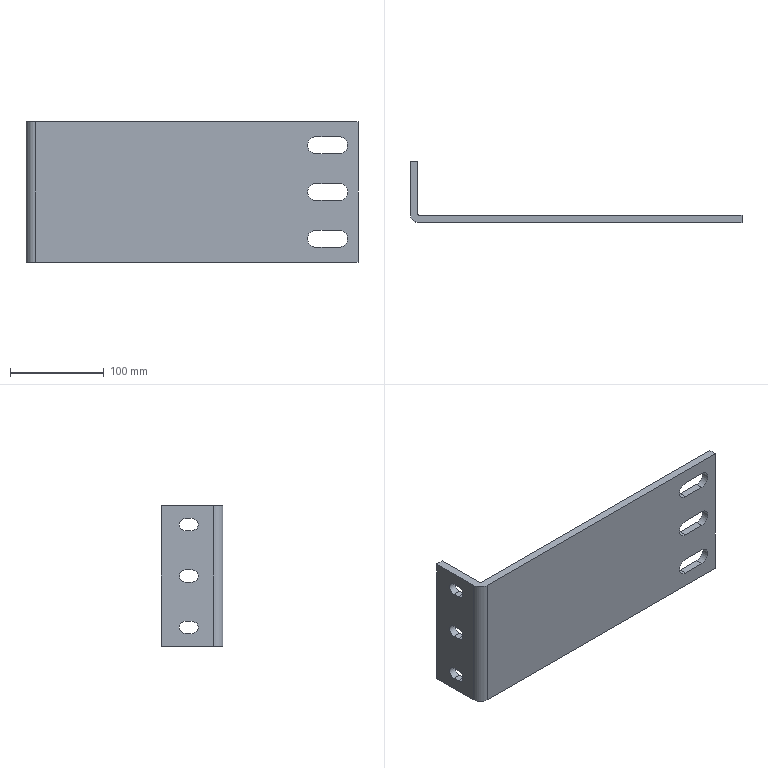Part | SolidWorks | features ICE 2, Extrusion 1 | 1 solid | 34 faces | box 355 x 66 x 150 mm | volume 470233 mm3 | plane 20 | cylinder 14 | commonest cylinder face diameters 13 x6 18 x6 4 x1 20 x1
STEP:
#1=CARTESIAN_POINT('',(8.,0.,0.));
#2=VERTEX_POINT('',#1);
#3=CARTESIAN_POINT('',(0.,0.,0.));
#4=VERTEX_POINT('',#3);
#5=CARTESIAN_POINT('',(8.,0.,0.));
#6=DIRECTION('',(-1.,0.,0.));
#7=VECTOR('',#6,1000.);
#8=LINE('',#5,#7);
#9=EDGE_CURVE('',#2,#4,#8,.T.);
#10=ORIENTED_EDGE('',*,*,#9,.T.);
#11=CARTESIAN_POINT('',(0.,0.,150.));
#12=VERTEX_POINT('',#11);
#13=CARTESIAN_POINT('',(0.,0.,150.));
#14=DIRECTION('',(0.,0.,-1.));
#15=VECTOR('',#14,1000.);
#16=LINE('',#13,#15);
#17=EDGE_CURVE('',#12,#4,#16,.T.);
#18=ORIENTED_EDGE('',*,*,#17,.F.);
#19=CARTESIAN_POINT('',(8.,0.,150.));
#20=VERTEX_POINT('',#19);
#21=CARTESIAN_POINT('',(8.,0.,150.));
#22=DIRECTION('',(-1.,0.,0.));
#23=VECTOR('',#22,1000.);
#24=LINE('',#21,#23);
#25=EDGE_CURVE('',#20,#12,#24,.T.);
#26=ORIENTED_EDGE('',*,*,#25,.F.);
#27=CARTESIAN_POINT('',(8.,0.,150.));
#28=DIRECTION('',(0.,0.,-1.));
#29=VECTOR('',#28,1000.);
#30=LINE('',#27,#29);
#31=EDGE_CURVE('',#20,#2,#30,.T.);
#32=ORIENTED_EDGE('',*,*,#31,.T.);
#33=EDGE_LOOP('',(#10,#18,#26,#32));
#34=FACE_OUTER_BOUND('',#33,.T.);
#35=CARTESIAN_POINT('',(8.,0.,150.));
#36=DIRECTION('',(0.,-1.,0.));
#37=DIRECTION('',(0.,0.,-1.));
#38=AXIS2_PLACEMENT_3D('',#35,#36,#37);
#39=PLANE('',#38);
#40=ADVANCED_FACE('',(#34),#39,.F.);
#41=CARTESIAN_POINT('',(0.,-26.,13.5));
#42=VERTEX_POINT('',#41);
#43=CARTESIAN_POINT('',(0.,-33.,13.5));
#44=VERTEX_POINT('',#43);
#45=CARTESIAN_POINT('',(0.,-26.,13.5));
#46=DIRECTION('',(0.,-1.,0.));
#47=VECTOR('',#46,1000.);
#48=LINE('',#45,#47);
#49=EDGE_CURVE('',#42,#44,#48,.T.);
#50=ORIENTED_EDGE('',*,*,#49,.F.);
#51=CARTESIAN_POINT('',(0.,-26.,26.5));
#52=VERTEX_POINT('',#51);
#53=CARTESIAN_POINT('',(0.,-26.,20.));
#54=DIRECTION('',(-1.,0.,0.));
#55=DIRECTION('',(0.,0.,1.));
#56=AXIS2_PLACEMENT_3D('',#53,#54,#55);
#57=CIRCLE('',#56,6.5);
#58=EDGE_CURVE('',#52,#42,#57,.T.);
#59=ORIENTED_EDGE('',*,*,#58,.F.);
#60=CARTESIAN_POINT('',(0.,-33.,26.5));
#61=VERTEX_POINT('',#60);
#62=CARTESIAN_POINT('',(0.,-26.,26.5));
#63=DIRECTION('',(0.,1.,0.));
#64=VECTOR('',#63,1000.);
#65=LINE('',#62,#64);
#66=EDGE_CURVE('',#61,#52,#65,.T.);
#67=ORIENTED_EDGE('',*,*,#66,.F.);
#68=CARTESIAN_POINT('',(0.,-33.,20.));
#69=DIRECTION('',(-1.,0.,0.));
#70=DIRECTION('',(0.,0.,1.));
#71=AXIS2_PLACEMENT_3D('',#68,#69,#70);
#72=CIRCLE('',#71,6.5);
#73=EDGE_CURVE('',#44,#61,#72,.T.);
#74=ORIENTED_EDGE('',*,*,#73,.F.);
#75=EDGE_LOOP('',(#50,#59,#67,#74));
#76=FACE_BOUND('',#75,.T.);
#77=CARTESIAN_POINT('',(0.,-26.,68.5));
#78=VERTEX_POINT('',#77);
#79=CARTESIAN_POINT('',(0.,-33.,68.5));
#80=VERTEX_POINT('',#79);
#81=CARTESIAN_POINT('',(0.,-26.,68.5));
#82=DIRECTION('',(0.,-1.,0.));
#83=VECTOR('',#82,1000.);
#84=LINE('',#81,#83);
#85=EDGE_CURVE('',#78,#80,#84,.T.);
#86=ORIENTED_EDGE('',*,*,#85,.F.);
#87=CARTESIAN_POINT('',(0.,-26.,81.5));
#88=VERTEX_POINT('',#87);
#89=CARTESIAN_POINT('',(0.,-26.,75.));
#90=DIRECTION('',(-1.,0.,0.));
#91=DIRECTION('',(0.,0.,1.));
#92=AXIS2_PLACEMENT_3D('',#89,#90,#91);
#93=CIRCLE('',#92,6.5);
#94=EDGE_CURVE('',#88,#78,#93,.T.);
#95=ORIENTED_EDGE('',*,*,#94,.F.);
#96=CARTESIAN_POINT('',(0.,-33.,81.5));
#97=VERTEX_POINT('',#96);
#98=CARTESIAN_POINT('',(0.,-26.,81.5));
#99=DIRECTION('',(0.,1.,0.));
#100=VECTOR('',#99,1000.);
#101=LINE('',#98,#100);
#102=EDGE_CURVE('',#97,#88,#101,.T.);
#103=ORIENTED_EDGE('',*,*,#102,.F.);
#104=CARTESIAN_POINT('',(0.,-33.,75.));
#105=DIRECTION('',(-1.,0.,0.));
#106=DIRECTION('',(0.,0.,1.));
#107=AXIS2_PLACEMENT_3D('',#104,#105,#106);
#108=CIRCLE('',#107,6.5);
#109=EDGE_CURVE('',#80,#97,#108,.T.);
#110=ORIENTED_EDGE('',*,*,#109,.F.);
#111=EDGE_LOOP('',(#86,#95,#103,#110));
#112=FACE_BOUND('',#111,.T.);
#113=CARTESIAN_POINT('',(0.,-26.,123.5));
#114=VERTEX_POINT('',#113);
#115=CARTESIAN_POINT('',(0.,-33.,123.5));
#116=VERTEX_POINT('',#115);
#117=CARTESIAN_POINT('',(0.,-26.,123.5));
#118=DIRECTION('',(0.,-1.,0.));
#119=VECTOR('',#118,1000.);
#120=LINE('',#117,#119);
#121=EDGE_CURVE('',#114,#116,#120,.T.);
#122=ORIENTED_EDGE('',*,*,#121,.F.);
#123=CARTESIAN_POINT('',(0.,-26.,136.5));
#124=VERTEX_POINT('',#123);
#125=CARTESIAN_POINT('',(0.,-26.,130.));
#126=DIRECTION('',(-1.,0.,0.));
#127=DIRECTION('',(0.,0.,1.));
#128=AXIS2_PLACEMENT_3D('',#125,#126,#127);
#129=CIRCLE('',#128,6.5);
#130=EDGE_CURVE('',#124,#114,#129,.T.);
#131=ORIENTED_EDGE('',*,*,#130,.F.);
#132=CARTESIAN_POINT('',(0.,-33.,136.5));
#133=VERTEX_POINT('',#132);
#134=CARTESIAN_POINT('',(0.,-26.,136.5));
#135=DIRECTION('',(0.,1.,0.));
#136=VECTOR('',#135,1000.);
#137=LINE('',#134,#136);
#138=EDGE_CURVE('',#133,#124,#137,.T.);
#139=ORIENTED_EDGE('',*,*,#138,.F.);
#140=CARTESIAN_POINT('',(0.,-33.,130.));
#141=DIRECTION('',(-1.,0.,0.));
#142=DIRECTION('',(0.,0.,1.));
#143=AXIS2_PLACEMENT_3D('',#140,#141,#142);
#144=CIRCLE('',#143,6.5);
#145=EDGE_CURVE('',#116,#133,#144,.T.);
#146=ORIENTED_EDGE('',*,*,#145,.F.);
#147=EDGE_LOOP('',(#122,#131,#139,#146));
#148=FACE_BOUND('',#147,.T.);
#149=CARTESIAN_POINT('',(0.,-56.,0.));
#150=VERTEX_POINT('',#149);
#151=CARTESIAN_POINT('',(0.,0.,0.));
#152=DIRECTION('',(0.,-1.,0.));
#153=VECTOR('',#152,1000.);
#154=LINE('',#151,#153);
#155=EDGE_CURVE('',#4,#150,#154,.T.);
#156=ORIENTED_EDGE('',*,*,#155,.T.);
#157=CARTESIAN_POINT('',(0.,-56.,150.));
#158=VERTEX_POINT('',#157);
#159=CARTESIAN_POINT('',(0.,-56.,150.));
#160=DIRECTION('',(0.,0.,-1.));
#161=VECTOR('',#160,1000.);
#162=LINE('',#159,#161);
#163=EDGE_CURVE('',#158,#150,#162,.T.);
#164=ORIENTED_EDGE('',*,*,#163,.F.);
#165=CARTESIAN_POINT('',(0.,0.,150.));
#166=DIRECTION('',(0.,-1.,0.));
#167=VECTOR('',#166,1000.);
#168=LINE('',#165,#167);
#169=EDGE_CURVE('',#12,#158,#168,.T.);
#170=ORIENTED_EDGE('',*,*,#169,.F.);
#171=ORIENTED_EDGE('',*,*,#17,.T.);
#172=EDGE_LOOP('',(#156,#164,#170,#171));
#173=FACE_OUTER_BOUND('',#172,.T.);
#174=CARTESIAN_POINT('',(0.,0.,150.));
#175=DIRECTION('',(1.,0.,0.));
#176=DIRECTION('',(0.,0.,-1.));
#177=AXIS2_PLACEMENT_3D('',#174,#175,#176);
#178=PLANE('',#177);
#179=ADVANCED_FACE('',(#76,#112,#148,#173),#178,.F.);
#180=CARTESIAN_POINT('',(10.,-66.,0.));
#181=VERTEX_POINT('',#180);
#182=CARTESIAN_POINT('',(10.,-56.,0.));
#183=DIRECTION('',(0.,0.,1.));
#184=DIRECTION('',(1.,0.,0.));
#185=AXIS2_PLACEMENT_3D('',#182,#183,#184);
#186=CIRCLE('',#185,10.);
#187=EDGE_CURVE('',#150,#181,#186,.T.);
#188=ORIENTED_EDGE('',*,*,#187,.T.);
#189=CARTESIAN_POINT('',(10.,-66.,150.));
#190=VERTEX_POINT('',#189);
#191=CARTESIAN_POINT('',(10.,-66.,150.));
#192=DIRECTION('',(0.,0.,-1.));
#193=VECTOR('',#192,1000.);
#194=LINE('',#191,#193);
#195=EDGE_CURVE('',#190,#181,#194,.T.);
#196=ORIENTED_EDGE('',*,*,#195,.F.);
#197=CARTESIAN_POINT('',(10.,-56.,150.));
#198=DIRECTION('',(0.,0.,1.));
#199=DIRECTION('',(1.,0.,0.));
#200=AXIS2_PLACEMENT_3D('',#197,#198,#199);
#201=CIRCLE('',#200,10.);
#202=EDGE_CURVE('',#158,#190,#201,.T.);
#203=ORIENTED_EDGE('',*,*,#202,.F.);
#204=ORIENTED_EDGE('',*,*,#163,.T.);
#205=EDGE_LOOP('',(#188,#196,#203,#204));
#206=FACE_OUTER_BOUND('',#205,.T.);
#207=CARTESIAN_POINT('',(10.,-56.,150.));
#208=DIRECTION('',(0.,0.,-1.));
#209=DIRECTION('',(-1.,0.,0.));
#210=AXIS2_PLACEMENT_3D('',#207,#208,#209);
#211=CYLINDRICAL_SURFACE('',#210,10.);
#212=ADVANCED_FACE('',(#206),#211,.T.);
#213=CARTESIAN_POINT('',(335.,-66.,16.));
#214=VERTEX_POINT('',#213);
#215=CARTESIAN_POINT('',(310.,-66.,16.));
#216=VERTEX_POINT('',#215);
#217=CARTESIAN_POINT('',(10.,-66.,16.));
#218=DIRECTION('',(-1.,0.,0.));
#219=VECTOR('',#218,1000.);
#220=LINE('',#217,#219);
#221=EDGE_CURVE('',#214,#216,#220,.T.);
#222=ORIENTED_EDGE('',*,*,#221,.T.);
#223=CARTESIAN_POINT('',(310.,-66.,34.));
#224=VERTEX_POINT('',#223);
#225=CARTESIAN_POINT('',(310.,-66.,25.));
#226=DIRECTION('',(0.,1.,0.));
#227=DIRECTION('',(0.,0.,1.));
#228=AXIS2_PLACEMENT_3D('',#225,#226,#227);
#229=CIRCLE('',#228,9.);
#230=EDGE_CURVE('',#216,#224,#229,.T.);
#231=ORIENTED_EDGE('',*,*,#230,.T.);
#232=CARTESIAN_POINT('',(335.,-66.,34.));
#233=VERTEX_POINT('',#232);
#234=CARTESIAN_POINT('',(10.,-66.,34.));
#235=DIRECTION('',(1.,0.,0.));
#236=VECTOR('',#235,1000.);
#237=LINE('',#234,#236);
#238=EDGE_CURVE('',#224,#233,#237,.T.);
#239=ORIENTED_EDGE('',*,*,#238,.T.);
#240=CARTESIAN_POINT('',(335.,-66.,25.));
#241=DIRECTION('',(0.,1.,0.));
#242=DIRECTION('',(0.,0.,1.));
#243=AXIS2_PLACEMENT_3D('',#240,#241,#242);
#244=CIRCLE('',#243,9.);
#245=EDGE_CURVE('',#233,#214,#244,.T.);
#246=ORIENTED_EDGE('',*,*,#245,.T.);
#247=EDGE_LOOP('',(#222,#231,#239,#246));
#248=FACE_BOUND('',#247,.T.);
#249=CARTESIAN_POINT('',(335.,-66.,66.));
#250=VERTEX_POINT('',#249);
#251=CARTESIAN_POINT('',(310.,-66.,66.));
#252=VERTEX_POINT('',#251);
#253=CARTESIAN_POINT('',(10.,-66.,66.));
#254=DIRECTION('',(-1.,0.,0.));
#255=VECTOR('',#254,1000.);
#256=LINE('',#253,#255);
#257=EDGE_CURVE('',#250,#252,#256,.T.);
#258=ORIENTED_EDGE('',*,*,#257,.T.);
#259=CARTESIAN_POINT('',(310.,-66.,84.));
#260=VERTEX_POINT('',#259);
#261=CARTESIAN_POINT('',(310.,-66.,75.));
#262=DIRECTION('',(0.,1.,0.));
#263=DIRECTION('',(0.,0.,1.));
#264=AXIS2_PLACEMENT_3D('',#261,#262,#263);
#265=CIRCLE('',#264,9.);
#266=EDGE_CURVE('',#252,#260,#265,.T.);
#267=ORIENTED_EDGE('',*,*,#266,.T.);
#268=CARTESIAN_POINT('',(335.,-66.,84.));
#269=VERTEX_POINT('',#268);
#270=CARTESIAN_POINT('',(10.,-66.,84.));
#271=DIRECTION('',(1.,0.,0.));
#272=VECTOR('',#271,1000.);
#273=LINE('',#270,#272);
#274=EDGE_CURVE('',#260,#269,#273,.T.);
#275=ORIENTED_EDGE('',*,*,#274,.T.);
#276=CARTESIAN_POINT('',(335.,-66.,75.));
#277=DIRECTION('',(0.,1.,0.));
#278=DIRECTION('',(0.,0.,1.));
#279=AXIS2_PLACEMENT_3D('',#276,#277,#278);
#280=CIRCLE('',#279,9.);
#281=EDGE_CURVE('',#269,#250,#280,.T.);
#282=ORIENTED_EDGE('',*,*,#281,.T.);
#283=EDGE_LOOP('',(#258,#267,#275,#282));
#284=FACE_BOUND('',#283,.T.);
#285=CARTESIAN_POINT('',(335.,-66.,116.));
#286=VERTEX_POINT('',#285);
#287=CARTESIAN_POINT('',(310.,-66.,116.));
#288=VERTEX_POINT('',#287);
#289=CARTESIAN_POINT('',(10.,-66.,116.));
#290=DIRECTION('',(-1.,0.,0.));
#291=VECTOR('',#290,1000.);
#292=LINE('',#289,#291);
#293=EDGE_CURVE('',#286,#288,#292,.T.);
#294=ORIENTED_EDGE('',*,*,#293,.T.);
#295=CARTESIAN_POINT('',(310.,-66.,134.));
#296=VERTEX_POINT('',#295);
#297=CARTESIAN_POINT('',(310.,-66.,125.));
#298=DIRECTION('',(0.,1.,0.));
#299=DIRECTION('',(0.,0.,1.));
#300=AXIS2_PLACEMENT_3D('',#297,#298,#299);
#301=CIRCLE('',#300,9.);
#302=EDGE_CURVE('',#288,#296,#301,.T.);
#303=ORIENTED_EDGE('',*,*,#302,.T.);
#304=CARTESIAN_POINT('',(335.,-66.,134.));
#305=VERTEX_POINT('',#304);
#306=CARTESIAN_POINT('',(10.,-66.,134.));
#307=DIRECTION('',(1.,0.,0.));
#308=VECTOR('',#307,1000.);
#309=LINE('',#306,#308);
#310=EDGE_CURVE('',#296,#305,#309,.T.);
#311=ORIENTED_EDGE('',*,*,#310,.T.);
#312=CARTESIAN_POINT('',(335.,-66.,125.));
#313=DIRECTION('',(0.,1.,0.));
#314=DIRECTION('',(0.,0.,1.));
#315=AXIS2_PLACEMENT_3D('',#312,#313,#314);
#316=CIRCLE('',#315,9.);
#317=EDGE_CURVE('',#305,#286,#316,.T.);
#318=ORIENTED_EDGE('',*,*,#317,.T.);
#319=EDGE_LOOP('',(#294,#303,#311,#318));
#320=FACE_BOUND('',#319,.T.);
#321=CARTESIAN_POINT('',(355.,-66.,0.));
#322=VERTEX_POINT('',#321);
#323=CARTESIAN_POINT('',(10.,-66.,0.));
#324=DIRECTION('',(1.,0.,0.));
#325=VECTOR('',#324,1000.);
#326=LINE('',#323,#325);
#327=EDGE_CURVE('',#181,#322,#326,.T.);
#328=ORIENTED_EDGE('',*,*,#327,.T.);
#329=CARTESIAN_POINT('',(355.,-66.,150.));
#330=VERTEX_POINT('',#329);
#331=CARTESIAN_POINT('',(355.,-66.,150.));
#332=DIRECTION('',(0.,0.,-1.));
#333=VECTOR('',#332,1000.);
#334=LINE('',#331,#333);
#335=EDGE_CURVE('',#330,#322,#334,.T.);
#336=ORIENTED_EDGE('',*,*,#335,.F.);
#337=CARTESIAN_POINT('',(10.,-66.,150.));
#338=DIRECTION('',(1.,0.,0.));
#339=VECTOR('',#338,1000.);
#340=LINE('',#337,#339);
#341=EDGE_CURVE('',#190,#330,#340,.T.);
#342=ORIENTED_EDGE('',*,*,#341,.F.);
#343=ORIENTED_EDGE('',*,*,#195,.T.);
#344=EDGE_LOOP('',(#328,#336,#342,#343));
#345=FACE_OUTER_BOUND('',#344,.T.);
#346=CARTESIAN_POINT('',(10.,-66.,150.));
#347=DIRECTION('',(0.,1.,0.));
#348=DIRECTION('',(0.,0.,1.));
#349=AXIS2_PLACEMENT_3D('',#346,#347,#348);
#350=PLANE('',#349);
#351=ADVANCED_FACE('',(#248,#284,#320,#345),#350,.F.);
#352=CARTESIAN_POINT('',(355.,-58.,0.));
#353=VERTEX_POINT('',#352);
#354=CARTESIAN_POINT('',(355.,-58.,0.));
#355=DIRECTION('',(0.,1.,0.));
#356=VECTOR('',#355,1000.);
#357=LINE('',#354,#356);
#358=EDGE_CURVE('',#322,#353,#357,.T.);
#359=ORIENTED_EDGE('',*,*,#358,.T.);
#360=CARTESIAN_POINT('',(355.,-58.,150.));
#361=VERTEX_POINT('',#360);
#362=CARTESIAN_POINT('',(355.,-58.,150.));
#363=DIRECTION('',(0.,0.,-1.));
#364=VECTOR('',#363,1000.);
#365=LINE('',#362,#364);
#366=EDGE_CURVE('',#361,#353,#365,.T.);
#367=ORIENTED_EDGE('',*,*,#366,.F.);
#368=CARTESIAN_POINT('',(355.,-58.,150.));
#369=DIRECTION('',(0.,1.,0.));
#370=VECTOR('',#369,1000.);
#371=LINE('',#368,#370);
#372=EDGE_CURVE('',#330,#361,#371,.T.);
#373=ORIENTED_EDGE('',*,*,#372,.F.);
#374=ORIENTED_EDGE('',*,*,#335,.T.);
#375=EDGE_LOOP('',(#359,#367,#373,#374));
#376=FACE_OUTER_BOUND('',#375,.T.);
#377=CARTESIAN_POINT('',(355.,-58.,150.));
#378=DIRECTION('',(-1.,0.,0.));
#379=DIRECTION('',(0.,0.,1.));
#380=AXIS2_PLACEMENT_3D('',#377,#378,#379);
#381=PLANE('',#380);
#382=ADVANCED_FACE('',(#376),#381,.F.);
#383=CARTESIAN_POINT('',(310.,-58.,34.));
#384=VERTEX_POINT('',#383);
#385=CARTESIAN_POINT('',(335.,-58.,34.));
#386=VERTEX_POINT('',#385);
#387=CARTESIAN_POINT('',(310.,-58.,34.));
#388=DIRECTION('',(1.,0.,0.));
#389=VECTOR('',#388,1000.);
#390=LINE('',#387,#389);
#391=EDGE_CURVE('',#384,#386,#390,.T.);
#392=ORIENTED_EDGE('',*,*,#391,.F.);
#393=CARTESIAN_POINT('',(310.,-58.,16.));
#394=VERTEX_POINT('',#393);
#395=CARTESIAN_POINT('',(310.,-58.,25.));
#396=DIRECTION('',(0.,1.,0.));
#397=DIRECTION('',(0.,0.,1.));
#398=AXIS2_PLACEMENT_3D('',#395,#396,#397);
#399=CIRCLE('',#398,9.);
#400=EDGE_CURVE('',#394,#384,#399,.T.);
#401=ORIENTED_EDGE('',*,*,#400,.F.);
#402=CARTESIAN_POINT('',(335.,-58.,16.));
#403=VERTEX_POINT('',#402);
#404=CARTESIAN_POINT('',(310.,-58.,16.));
#405=DIRECTION('',(-1.,0.,0.));
#406=VECTOR('',#405,1000.);
#407=LINE('',#404,#406);
#408=EDGE_CURVE('',#403,#394,#407,.T.);
#409=ORIENTED_EDGE('',*,*,#408,.F.);
#410=CARTESIAN_POINT('',(335.,-58.,25.));
#411=DIRECTION('',(0.,1.,0.));
#412=DIRECTION('',(0.,0.,1.));
#413=AXIS2_PLACEMENT_3D('',#410,#411,#412);
#414=CIRCLE('',#413,9.);
#415=EDGE_CURVE('',#386,#403,#414,.T.);
#416=ORIENTED_EDGE('',*,*,#415,.F.);
#417=EDGE_LOOP('',(#392,#401,#409,#416));
#418=FACE_BOUND('',#417,.T.);
#419=CARTESIAN_POINT('',(310.,-58.,84.));
#420=VERTEX_POINT('',#419);
#421=CARTESIAN_POINT('',(335.,-58.,84.));
#422=VERTEX_POINT('',#421);
#423=CARTESIAN_POINT('',(310.,-58.,84.));
#424=DIRECTION('',(1.,0.,0.));
#425=VECTOR('',#424,1000.);
#426=LINE('',#423,#425);
#427=EDGE_CURVE('',#420,#422,#426,.T.);
#428=ORIENTED_EDGE('',*,*,#427,.F.);
#429=CARTESIAN_POINT('',(310.,-58.,66.));
#430=VERTEX_POINT('',#429);
#431=CARTESIAN_POINT('',(310.,-58.,75.));
#432=DIRECTION('',(0.,1.,0.));
#433=DIRECTION('',(0.,0.,1.));
#434=AXIS2_PLACEMENT_3D('',#431,#432,#433);
#435=CIRCLE('',#434,9.);
#436=EDGE_CURVE('',#430,#420,#435,.T.);
#437=ORIENTED_EDGE('',*,*,#436,.F.);
#438=CARTESIAN_POINT('',(335.,-58.,66.));
#439=VERTEX_POINT('',#438);
#440=CARTESIAN_POINT('',(310.,-58.,66.));
#441=DIRECTION('',(-1.,0.,0.));
#442=VECTOR('',#441,1000.);
#443=LINE('',#440,#442);
#444=EDGE_CURVE('',#439,#430,#443,.T.);
#445=ORIENTED_EDGE('',*,*,#444,.F.);
#446=CARTESIAN_POINT('',(335.,-58.,75.));
#447=DIRECTION('',(0.,1.,0.));
#448=DIRECTION('',(0.,0.,1.));
#449=AXIS2_PLACEMENT_3D('',#446,#447,#448);
#450=CIRCLE('',#449,9.);
#451=EDGE_CURVE('',#422,#439,#450,.T.);
#452=ORIENTED_EDGE('',*,*,#451,.F.);
#453=EDGE_LOOP('',(#428,#437,#445,#452));
#454=FACE_BOUND('',#453,.T.);
#455=CARTESIAN_POINT('',(310.,-58.,134.));
#456=VERTEX_POINT('',#455);
#457=CARTESIAN_POINT('',(335.,-58.,134.));
#458=VERTEX_POINT('',#457);
#459=CARTESIAN_POINT('',(310.,-58.,134.));
#460=DIRECTION('',(1.,0.,0.));
#461=VECTOR('',#460,1000.);
#462=LINE('',#459,#461);
#463=EDGE_CURVE('',#456,#458,#462,.T.);
#464=ORIENTED_EDGE('',*,*,#463,.F.);
#465=CARTESIAN_POINT('',(310.,-58.,116.));
#466=VERTEX_POINT('',#465);
#467=CARTESIAN_POINT('',(310.,-58.,125.));
#468=DIRECTION('',(0.,1.,0.));
#469=DIRECTION('',(0.,0.,1.));
#470=AXIS2_PLACEMENT_3D('',#467,#468,#469);
#471=CIRCLE('',#470,9.);
#472=EDGE_CURVE('',#466,#456,#471,.T.);
#473=ORIENTED_EDGE('',*,*,#472,.F.);
#474=CARTESIAN_POINT('',(335.,-58.,116.));
#475=VERTEX_POINT('',#474);
#476=CARTESIAN_POINT('',(310.,-58.,116.));
#477=DIRECTION('',(-1.,0.,0.));
#478=VECTOR('',#477,1000.);
#479=LINE('',#476,#478);
#480=EDGE_CURVE('',#475,#466,#479,.T.);
#481=ORIENTED_EDGE('',*,*,#480,.F.);
#482=CARTESIAN_POINT('',(335.,-58.,125.));
#483=DIRECTION('',(0.,1.,0.));
#484=DIRECTION('',(0.,0.,1.));
#485=AXIS2_PLACEMENT_3D('',#482,#483,#484);
#486=CIRCLE('',#485,9.);
#487=EDGE_CURVE('',#458,#475,#486,.T.);
#488=ORIENTED_EDGE('',*,*,#487,.F.);
#489=EDGE_LOOP('',(#464,#473,#481,#488));
#490=FACE_BOUND('',#489,.T.);
#491=CARTESIAN_POINT('',(10.,-58.,0.));
#492=VERTEX_POINT('',#491);
#493=CARTESIAN_POINT('',(10.,-58.,0.));
#494=DIRECTION('',(-1.,0.,0.));
#495=VECTOR('',#494,1000.);
#496=LINE('',#493,#495);
#497=EDGE_CURVE('',#353,#492,#496,.T.);
#498=ORIENTED_EDGE('',*,*,#497,.T.);
#499=CARTESIAN_POINT('',(10.,-58.,150.));
#500=VERTEX_POINT('',#499);
#501=CARTESIAN_POINT('',(10.,-58.,150.));
#502=DIRECTION('',(0.,0.,-1.));
#503=VECTOR('',#502,1000.);
#504=LINE('',#501,#503);
#505=EDGE_CURVE('',#500,#492,#504,.T.);
#506=ORIENTED_EDGE('',*,*,#505,.F.);
#507=CARTESIAN_POINT('',(10.,-58.,150.));
#508=DIRECTION('',(-1.,0.,0.));
#509=VECTOR('',#508,1000.);
#510=LINE('',#507,#509);
#511=EDGE_CURVE('',#361,#500,#510,.T.);
#512=ORIENTED_EDGE('',*,*,#511,.F.);
#513=ORIENTED_EDGE('',*,*,#366,.T.);
#514=EDGE_LOOP('',(#498,#506,#512,#513));
#515=FACE_OUTER_BOUND('',#514,.T.);
#516=CARTESIAN_POINT('',(10.,-58.,150.));
#517=DIRECTION('',(0.,-1.,0.));
#518=DIRECTION('',(0.,0.,-1.));
#519=AXIS2_PLACEMENT_3D('',#516,#517,#518);
#520=PLANE('',#519);
#521=ADVANCED_FACE('',(#418,#454,#490,#515),#520,.F.);
#522=CARTESIAN_POINT('',(8.,-56.,0.));
#523=VERTEX_POINT('',#522);
#524=CARTESIAN_POINT('',(10.,-56.,0.));
#525=DIRECTION('',(0.,0.,-1.));
#526=DIRECTION('',(1.,0.,0.));
#527=AXIS2_PLACEMENT_3D('',#524,#525,#526);
#528=CIRCLE('',#527,2.);
#529=EDGE_CURVE('',#492,#523,#528,.T.);
#530=ORIENTED_EDGE('',*,*,#529,.T.);
#531=CARTESIAN_POINT('',(8.,-56.,150.));
#532=VERTEX_POINT('',#531);
#533=CARTESIAN_POINT('',(8.,-56.,150.));
#534=DIRECTION('',(0.,0.,-1.));
#535=VECTOR('',#534,1000.);
#536=LINE('',#533,#535);
#537=EDGE_CURVE('',#532,#523,#536,.T.);
#538=ORIENTED_EDGE('',*,*,#537,.F.);
#539=CARTESIAN_POINT('',(10.,-56.,150.));
#540=DIRECTION('',(0.,0.,-1.));
#541=DIRECTION('',(1.,0.,0.));
#542=AXIS2_PLACEMENT_3D('',#539,#540,#541);
#543=CIRCLE('',#542,2.);
#544=EDGE_CURVE('',#500,#532,#543,.T.);
#545=ORIENTED_EDGE('',*,*,#544,.F.);
#546=ORIENTED_EDGE('',*,*,#505,.T.);
#547=EDGE_LOOP('',(#530,#538,#545,#546));
#548=FACE_OUTER_BOUND('',#547,.T.);
#549=CARTESIAN_POINT('',(10.,-56.,150.));
#550=DIRECTION('',(0.,0.,-1.));
#551=DIRECTION('',(-1.,0.,0.));
#552=AXIS2_PLACEMENT_3D('',#549,#550,#551);
#553=CYLINDRICAL_SURFACE('',#552,2.);
#554=ADVANCED_FACE('',(#548),#553,.F.);
#555=CARTESIAN_POINT('',(8.,-33.,26.5));
#556=VERTEX_POINT('',#555);
#557=CARTESIAN_POINT('',(8.,-26.,26.5));
#558=VERTEX_POINT('',#557);
#559=CARTESIAN_POINT('',(8.,0.,26.5));
#560=DIRECTION('',(0.,1.,0.));
#561=VECTOR('',#560,1000.);
#562=LINE('',#559,#561);
#563=EDGE_CURVE('',#556,#558,#562,.T.);
#564=ORIENTED_EDGE('',*,*,#563,.T.);
#565=CARTESIAN_POINT('',(8.,-26.,13.5));
#566=VERTEX_POINT('',#565);
#567=CARTESIAN_POINT('',(8.,-26.,20.));
#568=DIRECTION('',(-1.,0.,0.));
#569=DIRECTION('',(0.,0.,1.));
#570=AXIS2_PLACEMENT_3D('',#567,#568,#569);
#571=CIRCLE('',#570,6.5);
#572=EDGE_CURVE('',#558,#566,#571,.T.);
#573=ORIENTED_EDGE('',*,*,#572,.T.);
#574=CARTESIAN_POINT('',(8.,-33.,13.5));
#575=VERTEX_POINT('',#574);
#576=CARTESIAN_POINT('',(8.,0.,13.5));
#577=DIRECTION('',(0.,-1.,0.));
#578=VECTOR('',#577,1000.);
#579=LINE('',#576,#578);
#580=EDGE_CURVE('',#566,#575,#579,.T.);
#581=ORIENTED_EDGE('',*,*,#580,.T.);
#582=CARTESIAN_POINT('',(8.,-33.,20.));
#583=DIRECTION('',(-1.,0.,0.));
#584=DIRECTION('',(0.,0.,1.));
#585=AXIS2_PLACEMENT_3D('',#582,#583,#584);
#586=CIRCLE('',#585,6.5);
#587=EDGE_CURVE('',#575,#556,#586,.T.);
#588=ORIENTED_EDGE('',*,*,#587,.T.);
#589=EDGE_LOOP('',(#564,#573,#581,#588));
#590=FACE_BOUND('',#589,.T.);
#591=CARTESIAN_POINT('',(8.,-33.,81.5));
#592=VERTEX_POINT('',#591);
#593=CARTESIAN_POINT('',(8.,-26.,81.5));
#594=VERTEX_POINT('',#593);
#595=CARTESIAN_POINT('',(8.,0.,81.5));
#596=DIRECTION('',(0.,1.,0.));
#597=VECTOR('',#596,1000.);
#598=LINE('',#595,#597);
#599=EDGE_CURVE('',#592,#594,#598,.T.);
#600=ORIENTED_EDGE('',*,*,#599,.T.);
#601=CARTESIAN_POINT('',(8.,-26.,68.5));
#602=VERTEX_POINT('',#601);
#603=CARTESIAN_POINT('',(8.,-26.,75.));
#604=DIRECTION('',(-1.,0.,0.));
#605=DIRECTION('',(0.,0.,1.));
#606=AXIS2_PLACEMENT_3D('',#603,#604,#605);
#607=CIRCLE('',#606,6.5);
#608=EDGE_CURVE('',#594,#602,#607,.T.);
#609=ORIENTED_EDGE('',*,*,#608,.T.);
#610=CARTESIAN_POINT('',(8.,-33.,68.5));
#611=VERTEX_POINT('',#610);
#612=CARTESIAN_POINT('',(8.,0.,68.5));
#613=DIRECTION('',(0.,-1.,0.));
#614=VECTOR('',#613,1000.);
#615=LINE('',#612,#614);
#616=EDGE_CURVE('',#602,#611,#615,.T.);
#617=ORIENTED_EDGE('',*,*,#616,.T.);
#618=CARTESIAN_POINT('',(8.,-33.,75.));
#619=DIRECTION('',(-1.,0.,0.));
#620=DIRECTION('',(0.,0.,1.));
#621=AXIS2_PLACEMENT_3D('',#618,#619,#620);
#622=CIRCLE('',#621,6.5);
#623=EDGE_CURVE('',#611,#592,#622,.T.);
#624=ORIENTED_EDGE('',*,*,#623,.T.);
#625=EDGE_LOOP('',(#600,#609,#617,#624));
#626=FACE_BOUND('',#625,.T.);
#627=CARTESIAN_POINT('',(8.,-33.,136.5));
#628=VERTEX_POINT('',#627);
#629=CARTESIAN_POINT('',(8.,-26.,136.5));
#630=VERTEX_POINT('',#629);
#631=CARTESIAN_POINT('',(8.,0.,136.5));
#632=DIRECTION('',(0.,1.,0.));
#633=VECTOR('',#632,1000.);
#634=LINE('',#631,#633);
#635=EDGE_CURVE('',#628,#630,#634,.T.);
#636=ORIENTED_EDGE('',*,*,#635,.T.);
#637=CARTESIAN_POINT('',(8.,-26.,123.5));
#638=VERTEX_POINT('',#637);
#639=CARTESIAN_POINT('',(8.,-26.,130.));
#640=DIRECTION('',(-1.,0.,0.));
#641=DIRECTION('',(0.,0.,1.));
#642=AXIS2_PLACEMENT_3D('',#639,#640,#641);
#643=CIRCLE('',#642,6.5);
#644=EDGE_CURVE('',#630,#638,#643,.T.);
#645=ORIENTED_EDGE('',*,*,#644,.T.);
#646=CARTESIAN_POINT('',(8.,-33.,123.5));
#647=VERTEX_POINT('',#646);
#648=CARTESIAN_POINT('',(8.,0.,123.5));
#649=DIRECTION('',(0.,-1.,0.));
#650=VECTOR('',#649,1000.);
#651=LINE('',#648,#650);
#652=EDGE_CURVE('',#638,#647,#651,.T.);
#653=ORIENTED_EDGE('',*,*,#652,.T.);
#654=CARTESIAN_POINT('',(8.,-33.,130.));
#655=DIRECTION('',(-1.,0.,0.));
#656=DIRECTION('',(0.,0.,1.));
#657=AXIS2_PLACEMENT_3D('',#654,#655,#656);
#658=CIRCLE('',#657,6.5);
#659=EDGE_CURVE('',#647,#628,#658,.T.);
#660=ORIENTED_EDGE('',*,*,#659,.T.);
#661=EDGE_LOOP('',(#636,#645,#653,#660));
#662=FACE_BOUND('',#661,.T.);
#663=CARTESIAN_POINT('',(8.,0.,0.));
#664=DIRECTION('',(0.,1.,0.));
#665=VECTOR('',#664,1000.);
#666=LINE('',#663,#665);
#667=EDGE_CURVE('',#523,#2,#666,.T.);
#668=ORIENTED_EDGE('',*,*,#667,.T.);
#669=ORIENTED_EDGE('',*,*,#31,.F.);
#670=CARTESIAN_POINT('',(8.,0.,150.));
#671=DIRECTION('',(0.,1.,0.));
#672=VECTOR('',#671,1000.);
#673=LINE('',#670,#672);
#674=EDGE_CURVE('',#532,#20,#673,.T.);
#675=ORIENTED_EDGE('',*,*,#674,.F.);
#676=ORIENTED_EDGE('',*,*,#537,.T.);
#677=EDGE_LOOP('',(#668,#669,#675,#676));
#678=FACE_OUTER_BOUND('',#677,.T.);
#679=CARTESIAN_POINT('',(8.,0.,150.));
#680=DIRECTION('',(-1.,0.,0.));
#681=DIRECTION('',(0.,0.,1.));
#682=AXIS2_PLACEMENT_3D('',#679,#680,#681);
#683=PLANE('',#682);
#684=ADVANCED_FACE('',(#590,#626,#662,#678),#683,.F.);
#685=ORIENTED_EDGE('',*,*,#25,.T.);
#686=ORIENTED_EDGE('',*,*,#169,.T.);
#687=ORIENTED_EDGE('',*,*,#202,.T.);
#688=ORIENTED_EDGE('',*,*,#341,.T.);
#689=ORIENTED_EDGE('',*,*,#372,.T.);
#690=ORIENTED_EDGE('',*,*,#511,.T.);
#691=ORIENTED_EDGE('',*,*,#544,.T.);
#692=ORIENTED_EDGE('',*,*,#674,.T.);
#693=EDGE_LOOP('',(#685,#686,#687,#688,#689,#690,#691,#692));
#694=FACE_OUTER_BOUND('',#693,.T.);
#695=CARTESIAN_POINT('',(10.,-56.,150.));
#696=DIRECTION('',(0.,0.,1.));
#697=DIRECTION('',(1.,0.,0.));
#698=AXIS2_PLACEMENT_3D('',#695,#696,#697);
#699=PLANE('',#698);
#700=ADVANCED_FACE('',(#694),#699,.T.);
#701=ORIENTED_EDGE('',*,*,#9,.F.);
#702=ORIENTED_EDGE('',*,*,#667,.F.);
#703=ORIENTED_EDGE('',*,*,#529,.F.);
#704=ORIENTED_EDGE('',*,*,#497,.F.);
#705=ORIENTED_EDGE('',*,*,#358,.F.);
#706=ORIENTED_EDGE('',*,*,#327,.F.);
#707=ORIENTED_EDGE('',*,*,#187,.F.);
#708=ORIENTED_EDGE('',*,*,#155,.F.);
#709=EDGE_LOOP('',(#701,#702,#703,#704,#705,#706,#707,#708));
#710=FACE_OUTER_BOUND('',#709,.T.);
#711=CARTESIAN_POINT('',(10.,-56.,0.));
#712=DIRECTION('',(0.,0.,1.));
#713=DIRECTION('',(1.,0.,0.));
#714=AXIS2_PLACEMENT_3D('',#711,#712,#713);
#715=PLANE('',#714);
#716=ADVANCED_FACE('',(#710),#715,.F.);
#717=CARTESIAN_POINT('',(150.,-26.,136.5));
#718=DIRECTION('',(-1.,0.,0.));
#719=VECTOR('',#718,1000.);
#720=LINE('',#717,#719);
#721=EDGE_CURVE('',#630,#124,#720,.T.);
#722=ORIENTED_EDGE('',*,*,#721,.T.);
#723=ORIENTED_EDGE('',*,*,#130,.T.);
#724=CARTESIAN_POINT('',(150.,-26.,123.5));
#725=DIRECTION('',(-1.,0.,0.));
#726=VECTOR('',#725,1000.);
#727=LINE('',#724,#726);
#728=EDGE_CURVE('',#638,#114,#727,.T.);
#729=ORIENTED_EDGE('',*,*,#728,.F.);
#730=ORIENTED_EDGE('',*,*,#644,.F.);
#731=EDGE_LOOP('',(#722,#723,#729,#730));
#732=FACE_OUTER_BOUND('',#731,.T.);
#733=CARTESIAN_POINT('',(150.,-26.,130.));
#734=DIRECTION('',(-1.,0.,0.));
#735=DIRECTION('',(0.,0.,1.));
#736=AXIS2_PLACEMENT_3D('',#733,#734,#735);
#737=CYLINDRICAL_SURFACE('',#736,6.5);
#738=ADVANCED_FACE('',(#732),#737,.F.);
#739=CARTESIAN_POINT('',(150.,-33.,136.5));
#740=DIRECTION('',(-1.,0.,0.));
#741=VECTOR('',#740,1000.);
#742=LINE('',#739,#741);
#743=EDGE_CURVE('',#628,#133,#742,.T.);
#744=ORIENTED_EDGE('',*,*,#743,.T.);
#745=ORIENTED_EDGE('',*,*,#138,.T.);
#746=ORIENTED_EDGE('',*,*,#721,.F.);
#747=ORIENTED_EDGE('',*,*,#635,.F.);
#748=EDGE_LOOP('',(#744,#745,#746,#747));
#749=FACE_OUTER_BOUND('',#748,.T.);
#750=CARTESIAN_POINT('',(150.,-26.,136.5));
#751=DIRECTION('',(0.,0.,1.));
#752=DIRECTION('',(1.,0.,0.));
#753=AXIS2_PLACEMENT_3D('',#750,#751,#752);
#754=PLANE('',#753);
#755=ADVANCED_FACE('',(#749),#754,.F.);
#756=CARTESIAN_POINT('',(150.,-33.,123.5));
#757=DIRECTION('',(-1.,0.,0.));
#758=VECTOR('',#757,1000.);
#759=LINE('',#756,#758);
#760=EDGE_CURVE('',#647,#116,#759,.T.);
#761=ORIENTED_EDGE('',*,*,#760,.T.);
#762=ORIENTED_EDGE('',*,*,#145,.T.);
#763=ORIENTED_EDGE('',*,*,#743,.F.);
#764=ORIENTED_EDGE('',*,*,#659,.F.);
#765=EDGE_LOOP('',(#761,#762,#763,#764));
#766=FACE_OUTER_BOUND('',#765,.T.);
#767=CARTESIAN_POINT('',(150.,-33.,130.));
#768=DIRECTION('',(-1.,0.,0.));
#769=DIRECTION('',(0.,0.,1.));
#770=AXIS2_PLACEMENT_3D('',#767,#768,#769);
#771=CYLINDRICAL_SURFACE('',#770,6.5);
#772=ADVANCED_FACE('',(#766),#771,.F.);
#773=ORIENTED_EDGE('',*,*,#728,.T.);
#774=ORIENTED_EDGE('',*,*,#121,.T.);
#775=ORIENTED_EDGE('',*,*,#760,.F.);
#776=ORIENTED_EDGE('',*,*,#652,.F.);
#777=EDGE_LOOP('',(#773,#774,#775,#776));
#778=FACE_OUTER_BOUND('',#777,.T.);
#779=CARTESIAN_POINT('',(150.,-26.,123.5));
#780=DIRECTION('',(0.,0.,-1.));
#781=DIRECTION('',(-1.,0.,0.));
#782=AXIS2_PLACEMENT_3D('',#779,#780,#781);
#783=PLANE('',#782);
#784=ADVANCED_FACE('',(#778),#783,.F.);
#785=CARTESIAN_POINT('',(150.,-26.,81.5));
#786=DIRECTION('',(-1.,0.,0.));
#787=VECTOR('',#786,1000.);
#788=LINE('',#785,#787);
#789=EDGE_CURVE('',#594,#88,#788,.T.);
#790=ORIENTED_EDGE('',*,*,#789,.T.);
#791=ORIENTED_EDGE('',*,*,#94,.T.);
#792=CARTESIAN_POINT('',(150.,-26.,68.5));
#793=DIRECTION('',(-1.,0.,0.));
#794=VECTOR('',#793,1000.);
#795=LINE('',#792,#794);
#796=EDGE_CURVE('',#602,#78,#795,.T.);
#797=ORIENTED_EDGE('',*,*,#796,.F.);
#798=ORIENTED_EDGE('',*,*,#608,.F.);
#799=EDGE_LOOP('',(#790,#791,#797,#798));
#800=FACE_OUTER_BOUND('',#799,.T.);
#801=CARTESIAN_POINT('',(150.,-26.,75.));
#802=DIRECTION('',(-1.,0.,0.));
#803=DIRECTION('',(0.,0.,1.));
#804=AXIS2_PLACEMENT_3D('',#801,#802,#803);
#805=CYLINDRICAL_SURFACE('',#804,6.5);
#806=ADVANCED_FACE('',(#800),#805,.F.);
#807=CARTESIAN_POINT('',(150.,-33.,81.5));
#808=DIRECTION('',(-1.,0.,0.));
#809=VECTOR('',#808,1000.);
#810=LINE('',#807,#809);
#811=EDGE_CURVE('',#592,#97,#810,.T.);
#812=ORIENTED_EDGE('',*,*,#811,.T.);
#813=ORIENTED_EDGE('',*,*,#102,.T.);
#814=ORIENTED_EDGE('',*,*,#789,.F.);
#815=ORIENTED_EDGE('',*,*,#599,.F.);
#816=EDGE_LOOP('',(#812,#813,#814,#815));
#817=FACE_OUTER_BOUND('',#816,.T.);
#818=CARTESIAN_POINT('',(150.,-26.,81.5));
#819=DIRECTION('',(0.,0.,1.));
#820=DIRECTION('',(1.,0.,0.));
#821=AXIS2_PLACEMENT_3D('',#818,#819,#820);
#822=PLANE('',#821);
#823=ADVANCED_FACE('',(#817),#822,.F.);
#824=CARTESIAN_POINT('',(150.,-33.,68.5));
#825=DIRECTION('',(-1.,0.,0.));
#826=VECTOR('',#825,1000.);
#827=LINE('',#824,#826);
#828=EDGE_CURVE('',#611,#80,#827,.T.);
#829=ORIENTED_EDGE('',*,*,#828,.T.);
#830=ORIENTED_EDGE('',*,*,#109,.T.);
#831=ORIENTED_EDGE('',*,*,#811,.F.);
#832=ORIENTED_EDGE('',*,*,#623,.F.);
#833=EDGE_LOOP('',(#829,#830,#831,#832));
#834=FACE_OUTER_BOUND('',#833,.T.);
#835=CARTESIAN_POINT('',(150.,-33.,75.));
#836=DIRECTION('',(-1.,0.,0.));
#837=DIRECTION('',(0.,0.,1.));
#838=AXIS2_PLACEMENT_3D('',#835,#836,#837);
#839=CYLINDRICAL_SURFACE('',#838,6.5);
#840=ADVANCED_FACE('',(#834),#839,.F.);
#841=ORIENTED_EDGE('',*,*,#796,.T.);
#842=ORIENTED_EDGE('',*,*,#85,.T.);
#843=ORIENTED_EDGE('',*,*,#828,.F.);
#844=ORIENTED_EDGE('',*,*,#616,.F.);
#845=EDGE_LOOP('',(#841,#842,#843,#844));
#846=FACE_OUTER_BOUND('',#845,.T.);
#847=CARTESIAN_POINT('',(150.,-26.,68.5));
#848=DIRECTION('',(0.,0.,-1.));
#849=DIRECTION('',(-1.,0.,0.));
#850=AXIS2_PLACEMENT_3D('',#847,#848,#849);
#851=PLANE('',#850);
#852=ADVANCED_FACE('',(#846),#851,.F.);
#853=CARTESIAN_POINT('',(150.,-26.,26.5));
#854=DIRECTION('',(-1.,0.,0.));
#855=VECTOR('',#854,1000.);
#856=LINE('',#853,#855);
#857=EDGE_CURVE('',#558,#52,#856,.T.);
#858=ORIENTED_EDGE('',*,*,#857,.T.);
#859=ORIENTED_EDGE('',*,*,#58,.T.);
#860=CARTESIAN_POINT('',(150.,-26.,13.5));
#861=DIRECTION('',(-1.,0.,0.));
#862=VECTOR('',#861,1000.);
#863=LINE('',#860,#862);
#864=EDGE_CURVE('',#566,#42,#863,.T.);
#865=ORIENTED_EDGE('',*,*,#864,.F.);
#866=ORIENTED_EDGE('',*,*,#572,.F.);
#867=EDGE_LOOP('',(#858,#859,#865,#866));
#868=FACE_OUTER_BOUND('',#867,.T.);
#869=CARTESIAN_POINT('',(150.,-26.,20.));
#870=DIRECTION('',(-1.,0.,0.));
#871=DIRECTION('',(0.,0.,1.));
#872=AXIS2_PLACEMENT_3D('',#869,#870,#871);
#873=CYLINDRICAL_SURFACE('',#872,6.5);
#874=ADVANCED_FACE('',(#868),#873,.F.);
#875=CARTESIAN_POINT('',(150.,-33.,26.5));
#876=DIRECTION('',(-1.,0.,0.));
#877=VECTOR('',#876,1000.);
#878=LINE('',#875,#877);
#879=EDGE_CURVE('',#556,#61,#878,.T.);
#880=ORIENTED_EDGE('',*,*,#879,.T.);
#881=ORIENTED_EDGE('',*,*,#66,.T.);
#882=ORIENTED_EDGE('',*,*,#857,.F.);
#883=ORIENTED_EDGE('',*,*,#563,.F.);
#884=EDGE_LOOP('',(#880,#881,#882,#883));
#885=FACE_OUTER_BOUND('',#884,.T.);
#886=CARTESIAN_POINT('',(150.,-26.,26.5));
#887=DIRECTION('',(0.,0.,1.));
#888=DIRECTION('',(1.,0.,0.));
#889=AXIS2_PLACEMENT_3D('',#886,#887,#888);
#890=PLANE('',#889);
#891=ADVANCED_FACE('',(#885),#890,.F.);
#892=CARTESIAN_POINT('',(150.,-33.,13.5));
#893=DIRECTION('',(-1.,0.,0.));
#894=VECTOR('',#893,1000.);
#895=LINE('',#892,#894);
#896=EDGE_CURVE('',#575,#44,#895,.T.);
#897=ORIENTED_EDGE('',*,*,#896,.T.);
#898=ORIENTED_EDGE('',*,*,#73,.T.);
#899=ORIENTED_EDGE('',*,*,#879,.F.);
#900=ORIENTED_EDGE('',*,*,#587,.F.);
#901=EDGE_LOOP('',(#897,#898,#899,#900));
#902=FACE_OUTER_BOUND('',#901,.T.);
#903=CARTESIAN_POINT('',(150.,-33.,20.));
#904=DIRECTION('',(-1.,0.,0.));
#905=DIRECTION('',(0.,0.,1.));
#906=AXIS2_PLACEMENT_3D('',#903,#904,#905);
#907=CYLINDRICAL_SURFACE('',#906,6.5);
#908=ADVANCED_FACE('',(#902),#907,.F.);
#909=ORIENTED_EDGE('',*,*,#864,.T.);
#910=ORIENTED_EDGE('',*,*,#49,.T.);
#911=ORIENTED_EDGE('',*,*,#896,.F.);
#912=ORIENTED_EDGE('',*,*,#580,.F.);
#913=EDGE_LOOP('',(#909,#910,#911,#912));
#914=FACE_OUTER_BOUND('',#913,.T.);
#915=CARTESIAN_POINT('',(150.,-26.,13.5));
#916=DIRECTION('',(0.,0.,-1.));
#917=DIRECTION('',(0.,1.,0.));
#918=AXIS2_PLACEMENT_3D('',#915,#916,#917);
#919=PLANE('',#918);
#920=ADVANCED_FACE('',(#914),#919,.F.);
#921=CARTESIAN_POINT('',(310.,-208.,116.));
#922=DIRECTION('',(0.,1.,0.));
#923=VECTOR('',#922,1000.);
#924=LINE('',#921,#923);
#925=EDGE_CURVE('',#288,#466,#924,.T.);
#926=ORIENTED_EDGE('',*,*,#925,.T.);
#927=ORIENTED_EDGE('',*,*,#472,.T.);
#928=CARTESIAN_POINT('',(310.,-208.,134.));
#929=DIRECTION('',(0.,1.,0.));
#930=VECTOR('',#929,1000.);
#931=LINE('',#928,#930);
#932=EDGE_CURVE('',#296,#456,#931,.T.);
#933=ORIENTED_EDGE('',*,*,#932,.F.);
#934=ORIENTED_EDGE('',*,*,#302,.F.);
#935=EDGE_LOOP('',(#926,#927,#933,#934));
#936=FACE_OUTER_BOUND('',#935,.T.);
#937=CARTESIAN_POINT('',(310.,-208.,125.));
#938=DIRECTION('',(0.,1.,0.));
#939=DIRECTION('',(0.,0.,1.));
#940=AXIS2_PLACEMENT_3D('',#937,#938,#939);
#941=CYLINDRICAL_SURFACE('',#940,9.);
#942=ADVANCED_FACE('',(#936),#941,.F.);
#943=CARTESIAN_POINT('',(335.,-208.,116.));
#944=DIRECTION('',(0.,1.,0.));
#945=VECTOR('',#944,1000.);
#946=LINE('',#943,#945);
#947=EDGE_CURVE('',#286,#475,#946,.T.);
#948=ORIENTED_EDGE('',*,*,#947,.T.);
#949=ORIENTED_EDGE('',*,*,#480,.T.);
#950=ORIENTED_EDGE('',*,*,#925,.F.);
#951=ORIENTED_EDGE('',*,*,#293,.F.);
#952=EDGE_LOOP('',(#948,#949,#950,#951));
#953=FACE_OUTER_BOUND('',#952,.T.);
#954=CARTESIAN_POINT('',(310.,-208.,116.));
#955=DIRECTION('',(0.,0.,-1.));
#956=DIRECTION('',(-1.,0.,0.));
#957=AXIS2_PLACEMENT_3D('',#954,#955,#956);
#958=PLANE('',#957);
#959=ADVANCED_FACE('',(#953),#958,.F.);
#960=CARTESIAN_POINT('',(335.,-208.,134.));
#961=DIRECTION('',(0.,1.,0.));
#962=VECTOR('',#961,1000.);
#963=LINE('',#960,#962);
#964=EDGE_CURVE('',#305,#458,#963,.T.);
#965=ORIENTED_EDGE('',*,*,#964,.T.);
#966=ORIENTED_EDGE('',*,*,#487,.T.);
#967=ORIENTED_EDGE('',*,*,#947,.F.);
#968=ORIENTED_EDGE('',*,*,#317,.F.);
#969=EDGE_LOOP('',(#965,#966,#967,#968));
#970=FACE_OUTER_BOUND('',#969,.T.);
#971=CARTESIAN_POINT('',(335.,-208.,125.));
#972=DIRECTION('',(0.,1.,0.));
#973=DIRECTION('',(0.,0.,1.));
#974=AXIS2_PLACEMENT_3D('',#971,#972,#973);
#975=CYLINDRICAL_SURFACE('',#974,9.);
#976=ADVANCED_FACE('',(#970),#975,.F.);
#977=ORIENTED_EDGE('',*,*,#932,.T.);
#978=ORIENTED_EDGE('',*,*,#463,.T.);
#979=ORIENTED_EDGE('',*,*,#964,.F.);
#980=ORIENTED_EDGE('',*,*,#310,.F.);
#981=EDGE_LOOP('',(#977,#978,#979,#980));
#982=FACE_OUTER_BOUND('',#981,.T.);
#983=CARTESIAN_POINT('',(310.,-208.,134.));
#984=DIRECTION('',(0.,0.,1.));
#985=DIRECTION('',(1.,0.,0.));
#986=AXIS2_PLACEMENT_3D('',#983,#984,#985);
#987=PLANE('',#986);
#988=ADVANCED_FACE('',(#982),#987,.F.);
#989=CARTESIAN_POINT('',(310.,-208.,66.));
#990=DIRECTION('',(0.,1.,0.));
#991=VECTOR('',#990,1000.);
#992=LINE('',#989,#991);
#993=EDGE_CURVE('',#252,#430,#992,.T.);
#994=ORIENTED_EDGE('',*,*,#993,.T.);
#995=ORIENTED_EDGE('',*,*,#436,.T.);
#996=CARTESIAN_POINT('',(310.,-208.,84.));
#997=DIRECTION('',(0.,1.,0.));
#998=VECTOR('',#997,1000.);
#999=LINE('',#996,#998);
#1000=EDGE_CURVE('',#260,#420,#999,.T.);
#1001=ORIENTED_EDGE('',*,*,#1000,.F.);
#1002=ORIENTED_EDGE('',*,*,#266,.F.);
#1003=EDGE_LOOP('',(#994,#995,#1001,#1002));
#1004=FACE_OUTER_BOUND('',#1003,.T.);
#1005=CARTESIAN_POINT('',(310.,-208.,75.));
#1006=DIRECTION('',(0.,1.,0.));
#1007=DIRECTION('',(0.,0.,1.));
#1008=AXIS2_PLACEMENT_3D('',#1005,#1006,#1007);
#1009=CYLINDRICAL_SURFACE('',#1008,9.);
#1010=ADVANCED_FACE('',(#1004),#1009,.F.);
#1011=CARTESIAN_POINT('',(335.,-208.,66.));
#1012=DIRECTION('',(0.,1.,0.));
#1013=VECTOR('',#1012,1000.);
#1014=LINE('',#1011,#1013);
#1015=EDGE_CURVE('',#250,#439,#1014,.T.);
#1016=ORIENTED_EDGE('',*,*,#1015,.T.);
#1017=ORIENTED_EDGE('',*,*,#444,.T.);
#1018=ORIENTED_EDGE('',*,*,#993,.F.);
#1019=ORIENTED_EDGE('',*,*,#257,.F.);
#1020=EDGE_LOOP('',(#1016,#1017,#1018,#1019));
#1021=FACE_OUTER_BOUND('',#1020,.T.);
#1022=CARTESIAN_POINT('',(310.,-208.,66.));
#1023=DIRECTION('',(0.,0.,-1.));
#1024=DIRECTION('',(-1.,0.,0.));
#1025=AXIS2_PLACEMENT_3D('',#1022,#1023,#1024);
#1026=PLANE('',#1025);
#1027=ADVANCED_FACE('',(#1021),#1026,.F.);
#1028=CARTESIAN_POINT('',(335.,-208.,84.));
#1029=DIRECTION('',(0.,1.,0.));
#1030=VECTOR('',#1029,1000.);
#1031=LINE('',#1028,#1030);
#1032=EDGE_CURVE('',#269,#422,#1031,.T.);
#1033=ORIENTED_EDGE('',*,*,#1032,.T.);
#1034=ORIENTED_EDGE('',*,*,#451,.T.);
#1035=ORIENTED_EDGE('',*,*,#1015,.F.);
#1036=ORIENTED_EDGE('',*,*,#281,.F.);
#1037=EDGE_LOOP('',(#1033,#1034,#1035,#1036));
#1038=FACE_OUTER_BOUND('',#1037,.T.);
#1039=CARTESIAN_POINT('',(335.,-208.,75.));
#1040=DIRECTION('',(0.,1.,0.));
#1041=DIRECTION('',(0.,0.,1.));
#1042=AXIS2_PLACEMENT_3D('',#1039,#1040,#1041);
#1043=CYLINDRICAL_SURFACE('',#1042,9.);
#1044=ADVANCED_FACE('',(#1038),#1043,.F.);
#1045=ORIENTED_EDGE('',*,*,#1000,.T.);
#1046=ORIENTED_EDGE('',*,*,#427,.T.);
#1047=ORIENTED_EDGE('',*,*,#1032,.F.);
#1048=ORIENTED_EDGE('',*,*,#274,.F.);
#1049=EDGE_LOOP('',(#1045,#1046,#1047,#1048));
#1050=FACE_OUTER_BOUND('',#1049,.T.);
#1051=CARTESIAN_POINT('',(310.,-208.,84.));
#1052=DIRECTION('',(0.,0.,1.));
#1053=DIRECTION('',(1.,0.,0.));
#1054=AXIS2_PLACEMENT_3D('',#1051,#1052,#1053);
#1055=PLANE('',#1054);
#1056=ADVANCED_FACE('',(#1050),#1055,.F.);
#1057=CARTESIAN_POINT('',(310.,-208.,16.));
#1058=DIRECTION('',(0.,1.,0.));
#1059=VECTOR('',#1058,1000.);
#1060=LINE('',#1057,#1059);
#1061=EDGE_CURVE('',#216,#394,#1060,.T.);
#1062=ORIENTED_EDGE('',*,*,#1061,.T.);
#1063=ORIENTED_EDGE('',*,*,#400,.T.);
#1064=CARTESIAN_POINT('',(310.,-208.,34.));
#1065=DIRECTION('',(0.,1.,0.));
#1066=VECTOR('',#1065,1000.);
#1067=LINE('',#1064,#1066);
#1068=EDGE_CURVE('',#224,#384,#1067,.T.);
#1069=ORIENTED_EDGE('',*,*,#1068,.F.);
#1070=ORIENTED_EDGE('',*,*,#230,.F.);
#1071=EDGE_LOOP('',(#1062,#1063,#1069,#1070));
#1072=FACE_OUTER_BOUND('',#1071,.T.);
#1073=CARTESIAN_POINT('',(310.,-208.,25.));
#1074=DIRECTION('',(0.,1.,0.));
#1075=DIRECTION('',(0.,0.,1.));
#1076=AXIS2_PLACEMENT_3D('',#1073,#1074,#1075);
#1077=CYLINDRICAL_SURFACE('',#1076,9.);
#1078=ADVANCED_FACE('',(#1072),#1077,.F.);
#1079=CARTESIAN_POINT('',(335.,-208.,16.));
#1080=DIRECTION('',(0.,1.,0.));
#1081=VECTOR('',#1080,1000.);
#1082=LINE('',#1079,#1081);
#1083=EDGE_CURVE('',#214,#403,#1082,.T.);
#1084=ORIENTED_EDGE('',*,*,#1083,.T.);
#1085=ORIENTED_EDGE('',*,*,#408,.T.);
#1086=ORIENTED_EDGE('',*,*,#1061,.F.);
#1087=ORIENTED_EDGE('',*,*,#221,.F.);
#1088=EDGE_LOOP('',(#1084,#1085,#1086,#1087));
#1089=FACE_OUTER_BOUND('',#1088,.T.);
#1090=CARTESIAN_POINT('',(310.,-208.,16.));
#1091=DIRECTION('',(0.,0.,-1.));
#1092=DIRECTION('',(-1.,0.,0.));
#1093=AXIS2_PLACEMENT_3D('',#1090,#1091,#1092);
#1094=PLANE('',#1093);
#1095=ADVANCED_FACE('',(#1089),#1094,.F.);
#1096=CARTESIAN_POINT('',(335.,-208.,34.));
#1097=DIRECTION('',(0.,1.,0.));
#1098=VECTOR('',#1097,1000.);
#1099=LINE('',#1096,#1098);
#1100=EDGE_CURVE('',#233,#386,#1099,.T.);
#1101=ORIENTED_EDGE('',*,*,#1100,.T.);
#1102=ORIENTED_EDGE('',*,*,#415,.T.);
#1103=ORIENTED_EDGE('',*,*,#1083,.F.);
#1104=ORIENTED_EDGE('',*,*,#245,.F.);
#1105=EDGE_LOOP('',(#1101,#1102,#1103,#1104));
#1106=FACE_OUTER_BOUND('',#1105,.T.);
#1107=CARTESIAN_POINT('',(335.,-208.,25.));
#1108=DIRECTION('',(0.,1.,0.));
#1109=DIRECTION('',(0.,0.,1.));
#1110=AXIS2_PLACEMENT_3D('',#1107,#1108,#1109);
#1111=CYLINDRICAL_SURFACE('',#1110,9.);
#1112=ADVANCED_FACE('',(#1106),#1111,.F.);
#1113=ORIENTED_EDGE('',*,*,#1068,.T.);
#1114=ORIENTED_EDGE('',*,*,#391,.T.);
#1115=ORIENTED_EDGE('',*,*,#1100,.F.);
#1116=ORIENTED_EDGE('',*,*,#238,.F.);
#1117=EDGE_LOOP('',(#1113,#1114,#1115,#1116));
#1118=FACE_OUTER_BOUND('',#1117,.T.);
#1119=CARTESIAN_POINT('',(310.,-208.,34.));
#1120=DIRECTION('',(0.,0.,1.));
#1121=DIRECTION('',(1.,0.,0.));
#1122=AXIS2_PLACEMENT_3D('',#1119,#1120,#1121);
#1123=PLANE('',#1122);
#1124=ADVANCED_FACE('',(#1118),#1123,.F.);
#1125=CLOSED_SHELL('',(#40,#179,#212,#351,#382,#521,#554,#684,#700,#716,#738,#755,#772,#784,#806,#823,#840,#852,#874,#891,#908,#920,#942,#959,#976,#988,#1010,#1027,#1044,#1056,#1078,#1095,#1112,#1124));
#1126=MANIFOLD_SOLID_BREP('',#1125);
#1127=CARTESIAN_POINT('',(0.,0.,0.));
#1128=DIRECTION('',(0.,0.,1.));
#1129=DIRECTION('',(1.,0.,0.));
#1130=AXIS2_PLACEMENT_3D('',#1127,#1128,#1129);
#1131=(LENGTH_UNIT()NAMED_UNIT(*)SI_UNIT(.MILLI.,.METRE.));
#1132=UNCERTAINTY_MEASURE_WITH_UNIT(LENGTH_MEASURE(0.00001),#1131,'','');
#1133=(NAMED_UNIT(*)PLANE_ANGLE_UNIT()SI_UNIT($,.RADIAN.));
#1134=(NAMED_UNIT(*)SI_UNIT($,.STERADIAN.)SOLID_ANGLE_UNIT());
#1135=(GEOMETRIC_REPRESENTATION_CONTEXT(3)GLOBAL_UNCERTAINTY_ASSIGNED_CONTEXT((#1132))GLOBAL_UNIT_ASSIGNED_CONTEXT((#1131,#1133,#1134))REPRESENTATION_CONTEXT('',''));
#1136=ADVANCED_BREP_SHAPE_REPRESENTATION('',(#1126,#1130),#1135);